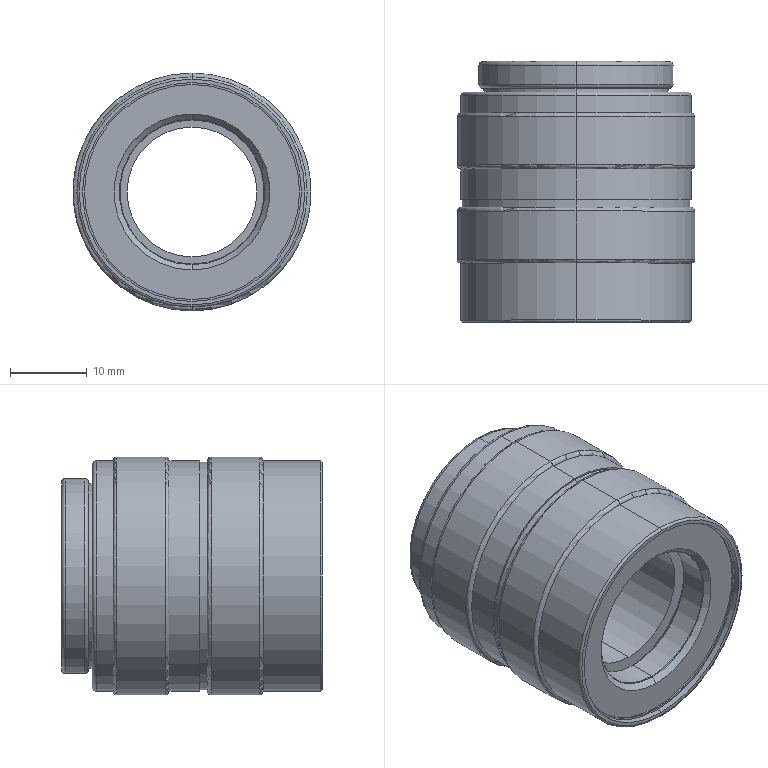Part | STEP file | LTABA30_LTABA30 | 1 solid | 66 faces | box 31 x 34 x 31 mm | volume 15140 mm3 | cylinder 32 | torus 16 | plane 12 | cone 6 | commonest cylinder face diameters 30 x6 31 x4 16.933 x2 18.786 x2 18.933 x2 21 x2